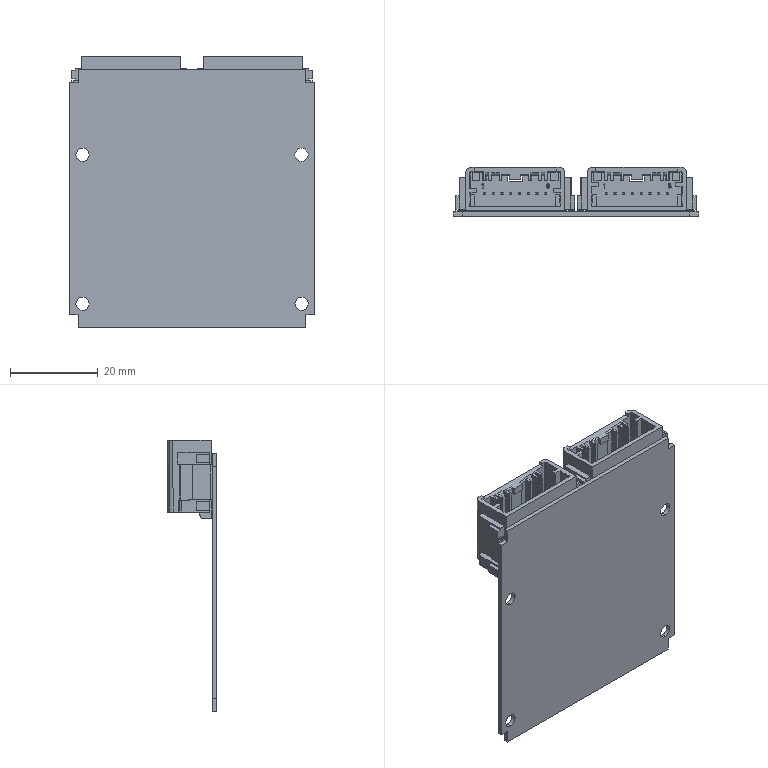Part | NX | features BREP 3 | 3 solids | 1316 faces | box 56 x 11.171 x 62 mm | volume 6321 mm3 | plane 1036 | cylinder 276 | spline 4 | commonest cylinder face diameters 0.4 x116 1.6 x40 0.6 x32 0.8 x32 1.2 x32 2.4 x8